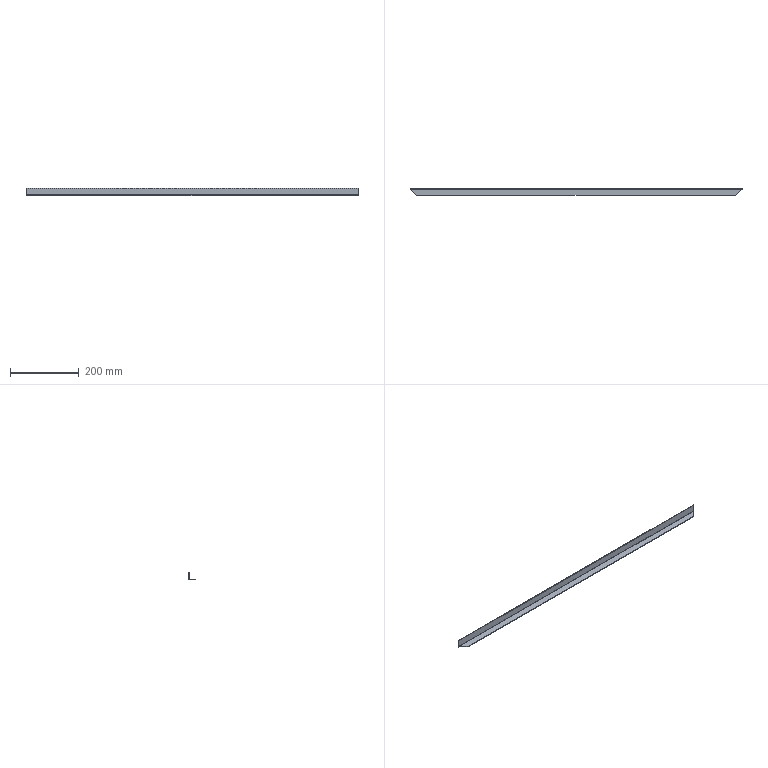Part | STEP file | Rear Closing Plate Frame Lower 1 | 1 solid | 22 faces | box 963 x 20 x 22 mm | volume 74999 mm3 | plane 18 | cylinder 2 | spline 2 | commonest cylinder face diameters 1 x1 5 x1
STEP:
#1=CARTESIAN_POINT('',(-1.251,219.392,2.5));
#2=VERTEX_POINT('',#1);
#3=CARTESIAN_POINT('',(957.749,219.392,2.5));
#4=VERTEX_POINT('',#3);
#5=CARTESIAN_POINT('',(-3.251,219.392,2.5));
#6=DIRECTION('',(1.,0.,0.));
#7=VECTOR('',#6,1000.);
#8=LINE('',#5,#7);
#9=EDGE_CURVE('',#2,#4,#8,.T.);
#10=ORIENTED_EDGE('',*,*,#9,.F.);
#11=CARTESIAN_POINT('',(-1.251,219.392,3.5));
#12=VERTEX_POINT('',#11);
#13=CARTESIAN_POINT('',(-1.251,219.392,22.));
#14=DIRECTION('',(0.,0.,1.));
#15=VECTOR('',#14,1000.);
#16=LINE('',#13,#15);
#17=EDGE_CURVE('',#2,#12,#16,.T.);
#18=ORIENTED_EDGE('',*,*,#17,.T.);
#19=CARTESIAN_POINT('',(-2.251,219.392,3.5));
#20=VERTEX_POINT('',#19);
#21=CARTESIAN_POINT('',(-3.251,219.392,3.5));
#22=DIRECTION('',(-1.,0.,0.));
#23=VECTOR('',#22,1000.);
#24=LINE('',#21,#23);
#25=EDGE_CURVE('',#12,#20,#24,.T.);
#26=ORIENTED_EDGE('',*,*,#25,.T.);
#27=CARTESIAN_POINT('',(-2.251,219.392,0.));
#28=VERTEX_POINT('',#27);
#29=CARTESIAN_POINT('',(-2.251,219.392,22.));
#30=DIRECTION('',(0.,0.,1.));
#31=VECTOR('',#30,1000.);
#32=LINE('',#29,#31);
#33=EDGE_CURVE('',#28,#20,#32,.T.);
#34=ORIENTED_EDGE('',*,*,#33,.F.);
#35=CARTESIAN_POINT('',(-3.251,219.392,0.));
#36=VERTEX_POINT('',#35);
#37=CARTESIAN_POINT('',(-3.251,219.392,0.));
#38=DIRECTION('',(1.,0.,0.));
#39=VECTOR('',#38,1000.);
#40=LINE('',#37,#39);
#41=EDGE_CURVE('',#36,#28,#40,.T.);
#42=ORIENTED_EDGE('',*,*,#41,.F.);
#43=CARTESIAN_POINT('',(-3.251,219.392,22.));
#44=VERTEX_POINT('',#43);
#45=CARTESIAN_POINT('',(-3.251,219.392,22.));
#46=DIRECTION('',(0.,0.,-1.));
#47=VECTOR('',#46,1000.);
#48=LINE('',#45,#47);
#49=EDGE_CURVE('',#44,#36,#48,.T.);
#50=ORIENTED_EDGE('',*,*,#49,.F.);
#51=CARTESIAN_POINT('',(959.749,219.392,22.));
#52=VERTEX_POINT('',#51);
#53=CARTESIAN_POINT('',(-3.251,219.392,22.));
#54=DIRECTION('',(-1.,0.,0.));
#55=VECTOR('',#54,1000.);
#56=LINE('',#53,#55);
#57=EDGE_CURVE('',#52,#44,#56,.T.);
#58=ORIENTED_EDGE('',*,*,#57,.F.);
#59=CARTESIAN_POINT('',(959.749,219.392,0.));
#60=VERTEX_POINT('',#59);
#61=CARTESIAN_POINT('',(959.749,219.392,22.));
#62=DIRECTION('',(0.,0.,1.));
#63=VECTOR('',#62,1000.);
#64=LINE('',#61,#63);
#65=EDGE_CURVE('',#60,#52,#64,.T.);
#66=ORIENTED_EDGE('',*,*,#65,.F.);
#67=CARTESIAN_POINT('',(958.749,219.392,0.));
#68=VERTEX_POINT('',#67);
#69=CARTESIAN_POINT('',(959.749,219.392,0.));
#70=DIRECTION('',(1.,0.,0.));
#71=VECTOR('',#70,1000.);
#72=LINE('',#69,#71);
#73=EDGE_CURVE('',#68,#60,#72,.T.);
#74=ORIENTED_EDGE('',*,*,#73,.F.);
#75=CARTESIAN_POINT('',(958.749,219.392,3.5));
#76=VERTEX_POINT('',#75);
#77=CARTESIAN_POINT('',(958.749,219.392,22.));
#78=DIRECTION('',(0.,0.,-1.));
#79=VECTOR('',#78,1000.);
#80=LINE('',#77,#79);
#81=EDGE_CURVE('',#76,#68,#80,.T.);
#82=ORIENTED_EDGE('',*,*,#81,.F.);
#83=CARTESIAN_POINT('',(957.749,219.392,3.5));
#84=VERTEX_POINT('',#83);
#85=CARTESIAN_POINT('',(-3.251,219.392,3.5));
#86=DIRECTION('',(-1.,0.,0.));
#87=VECTOR('',#86,1000.);
#88=LINE('',#85,#87);
#89=EDGE_CURVE('',#76,#84,#88,.T.);
#90=ORIENTED_EDGE('',*,*,#89,.T.);
#91=CARTESIAN_POINT('',(957.749,219.392,22.));
#92=DIRECTION('',(0.,0.,-1.));
#93=VECTOR('',#92,1000.);
#94=LINE('',#91,#93);
#95=EDGE_CURVE('',#84,#4,#94,.T.);
#96=ORIENTED_EDGE('',*,*,#95,.T.);
#97=EDGE_LOOP('',(#10,#18,#26,#34,#42,#50,#58,#66,#74,#82,#90,#96));
#98=FACE_OUTER_BOUND('',#97,.T.);
#99=CARTESIAN_POINT('',(-3.251,219.392,22.));
#100=DIRECTION('',(0.,-1.,0.));
#101=DIRECTION('',(1.,0.,0.));
#102=AXIS2_PLACEMENT_3D('',#99,#100,#101);
#103=PLANE('',#102);
#104=ADVANCED_FACE('',(#98),#103,.F.);
#105=CARTESIAN_POINT('',(957.749,218.142,0.3349));
#106=VERTEX_POINT('',#105);
#107=CARTESIAN_POINT('',(957.749,216.892,2.5));
#108=DIRECTION('',(-1.,0.,0.));
#109=DIRECTION('',(0.,0.,1.));
#110=AXIS2_PLACEMENT_3D('',#107,#108,#109);
#111=CIRCLE('',#110,2.5);
#112=EDGE_CURVE('',#4,#106,#111,.T.);
#113=ORIENTED_EDGE('',*,*,#112,.T.);
#114=CARTESIAN_POINT('',(957.249,216.892,0.));
#115=VERTEX_POINT('',#114);
#116=CARTESIAN_POINT('',(957.249,216.892,0.));
#117=CARTESIAN_POINT('',(957.332,217.11,0.));
#118=CARTESIAN_POINT('',(957.416,217.328,0.02876));
#119=CARTESIAN_POINT('',(957.583,217.751,0.1422));
#120=CARTESIAN_POINT('',(957.665,217.952,0.2255));
#121=CARTESIAN_POINT('',(957.749,218.142,0.3349));
#122=B_SPLINE_CURVE_WITH_KNOTS('',3,(#116,#117,#118,#119,#120,#121),.UNSPECIFIED.,.F.,.F.,(4,2,4),(0.,0.0007013,0.001403),.UNSPECIFIED.);
#123=EDGE_CURVE('',#115,#106,#122,.T.);
#124=ORIENTED_EDGE('',*,*,#123,.F.);
#125=CARTESIAN_POINT('',(-0.7512,216.892,0.));
#126=VERTEX_POINT('',#125);
#127=CARTESIAN_POINT('',(1921.52,216.892,0.));
#128=DIRECTION('',(-1.,0.,0.));
#129=VECTOR('',#128,1000.);
#130=LINE('',#127,#129);
#131=EDGE_CURVE('',#115,#126,#130,.T.);
#132=ORIENTED_EDGE('',*,*,#131,.T.);
#133=CARTESIAN_POINT('',(-1.251,218.142,0.3349));
#134=VERTEX_POINT('',#133);
#135=CARTESIAN_POINT('',(-1.251,218.142,0.3349));
#136=CARTESIAN_POINT('',(-1.168,217.952,0.2255));
#137=CARTESIAN_POINT('',(-1.084,217.749,0.1414));
#138=CARTESIAN_POINT('',(-0.9172,217.326,0.02839));
#139=CARTESIAN_POINT('',(-0.8347,217.11,0.));
#140=CARTESIAN_POINT('',(-0.7512,216.892,0.));
#141=B_SPLINE_CURVE_WITH_KNOTS('',3,(#135,#136,#137,#138,#139,#140),.UNSPECIFIED.,.F.,.F.,(4,2,4),(0.,0.0007013,0.001403),.UNSPECIFIED.);
#142=EDGE_CURVE('',#134,#126,#141,.T.);
#143=ORIENTED_EDGE('',*,*,#142,.F.);
#144=CARTESIAN_POINT('',(-1.251,216.892,2.5));
#145=DIRECTION('',(1.,0.,0.));
#146=DIRECTION('',(0.,0.,1.));
#147=AXIS2_PLACEMENT_3D('',#144,#145,#146);
#148=CIRCLE('',#147,2.5);
#149=EDGE_CURVE('',#134,#2,#148,.T.);
#150=ORIENTED_EDGE('',*,*,#149,.T.);
#151=ORIENTED_EDGE('',*,*,#9,.T.);
#152=EDGE_LOOP('',(#113,#124,#132,#143,#150,#151));
#153=FACE_OUTER_BOUND('',#152,.T.);
#154=CARTESIAN_POINT('',(1921.52,216.892,2.5));
#155=DIRECTION('',(-1.,0.,0.));
#156=DIRECTION('',(0.,0.,1.));
#157=AXIS2_PLACEMENT_3D('',#154,#155,#156);
#158=CYLINDRICAL_SURFACE('',#157,2.5);
#159=ADVANCED_FACE('',(#153),#158,.T.);
#160=ORIENTED_EDGE('',*,*,#33,.T.);
#161=CARTESIAN_POINT('',(-2.251,217.392,3.5));
#162=VERTEX_POINT('',#161);
#163=CARTESIAN_POINT('',(-2.251,-1709.111,3.5));
#164=DIRECTION('',(0.,1.,0.));
#165=VECTOR('',#164,1000.);
#166=LINE('',#163,#165);
#167=EDGE_CURVE('',#162,#20,#166,.T.);
#168=ORIENTED_EDGE('',*,*,#167,.F.);
#169=CARTESIAN_POINT('',(-2.251,217.392,0.));
#170=VERTEX_POINT('',#169);
#171=CARTESIAN_POINT('',(-2.251,217.392,22.));
#172=DIRECTION('',(0.,0.,1.));
#173=VECTOR('',#172,1000.);
#174=LINE('',#171,#173);
#175=EDGE_CURVE('',#170,#162,#174,.T.);
#176=ORIENTED_EDGE('',*,*,#175,.F.);
#177=CARTESIAN_POINT('',(-2.251,-1709.111,0.));
#178=DIRECTION('',(0.,-1.,0.));
#179=VECTOR('',#178,1000.);
#180=LINE('',#177,#179);
#181=EDGE_CURVE('',#28,#170,#180,.T.);
#182=ORIENTED_EDGE('',*,*,#181,.F.);
#183=EDGE_LOOP('',(#160,#168,#176,#182));
#184=FACE_OUTER_BOUND('',#183,.T.);
#185=CARTESIAN_POINT('',(-2.251,-1709.111,22.));
#186=DIRECTION('',(-1.,0.,0.));
#187=DIRECTION('',(0.,0.,1.));
#188=AXIS2_PLACEMENT_3D('',#185,#186,#187);
#189=PLANE('',#188);
#190=ADVANCED_FACE('',(#184),#189,.F.);
#191=ORIENTED_EDGE('',*,*,#49,.T.);
#192=CARTESIAN_POINT('',(-3.251,217.392,0.));
#193=VERTEX_POINT('',#192);
#194=CARTESIAN_POINT('',(-3.251,-1709.111,0.));
#195=DIRECTION('',(0.,1.,0.));
#196=VECTOR('',#195,1000.);
#197=LINE('',#194,#196);
#198=EDGE_CURVE('',#193,#36,#197,.T.);
#199=ORIENTED_EDGE('',*,*,#198,.F.);
#200=CARTESIAN_POINT('',(-3.251,217.392,22.));
#201=VERTEX_POINT('',#200);
#202=CARTESIAN_POINT('',(-3.251,217.392,22.));
#203=DIRECTION('',(0.,0.,-1.));
#204=VECTOR('',#203,1000.);
#205=LINE('',#202,#204);
#206=EDGE_CURVE('',#201,#193,#205,.T.);
#207=ORIENTED_EDGE('',*,*,#206,.F.);
#208=CARTESIAN_POINT('',(-3.251,-1709.111,22.));
#209=DIRECTION('',(0.,-1.,0.));
#210=VECTOR('',#209,1000.);
#211=LINE('',#208,#210);
#212=EDGE_CURVE('',#44,#201,#211,.T.);
#213=ORIENTED_EDGE('',*,*,#212,.F.);
#214=EDGE_LOOP('',(#191,#199,#207,#213));
#215=FACE_OUTER_BOUND('',#214,.T.);
#216=CARTESIAN_POINT('',(-3.251,-1709.111,22.));
#217=DIRECTION('',(1.,0.,0.));
#218=DIRECTION('',(0.,0.,-1.));
#219=AXIS2_PLACEMENT_3D('',#216,#217,#218);
#220=PLANE('',#219);
#221=ADVANCED_FACE('',(#215),#220,.F.);
#222=ORIENTED_EDGE('',*,*,#57,.T.);
#223=ORIENTED_EDGE('',*,*,#212,.T.);
#224=CARTESIAN_POINT('',(959.749,217.392,22.));
#225=VERTEX_POINT('',#224);
#226=CARTESIAN_POINT('',(0.,217.392,22.));
#227=DIRECTION('',(-1.,0.,0.));
#228=VECTOR('',#227,1000.);
#229=LINE('',#226,#228);
#230=EDGE_CURVE('',#225,#201,#229,.T.);
#231=ORIENTED_EDGE('',*,*,#230,.F.);
#232=CARTESIAN_POINT('',(959.749,-1709.111,22.));
#233=DIRECTION('',(0.,-1.,0.));
#234=VECTOR('',#233,1000.);
#235=LINE('',#232,#234);
#236=EDGE_CURVE('',#52,#225,#235,.T.);
#237=ORIENTED_EDGE('',*,*,#236,.F.);
#238=EDGE_LOOP('',(#222,#223,#231,#237));
#239=FACE_OUTER_BOUND('',#238,.T.);
#240=CARTESIAN_POINT('',(0.,-1709.111,22.));
#241=DIRECTION('',(0.,0.,-1.));
#242=DIRECTION('',(-1.,0.,0.));
#243=AXIS2_PLACEMENT_3D('',#240,#241,#242);
#244=PLANE('',#243);
#245=ADVANCED_FACE('',(#239),#244,.F.);
#246=CARTESIAN_POINT('',(959.749,217.392,0.));
#247=VERTEX_POINT('',#246);
#248=CARTESIAN_POINT('',(959.749,217.392,22.));
#249=DIRECTION('',(0.,0.,-1.));
#250=VECTOR('',#249,1000.);
#251=LINE('',#248,#250);
#252=EDGE_CURVE('',#225,#247,#251,.T.);
#253=ORIENTED_EDGE('',*,*,#252,.T.);
#254=CARTESIAN_POINT('',(959.749,-1709.111,0.));
#255=DIRECTION('',(0.,1.,0.));
#256=VECTOR('',#255,1000.);
#257=LINE('',#254,#256);
#258=EDGE_CURVE('',#247,#60,#257,.T.);
#259=ORIENTED_EDGE('',*,*,#258,.T.);
#260=ORIENTED_EDGE('',*,*,#65,.T.);
#261=ORIENTED_EDGE('',*,*,#236,.T.);
#262=EDGE_LOOP('',(#253,#259,#260,#261));
#263=FACE_OUTER_BOUND('',#262,.T.);
#264=CARTESIAN_POINT('',(959.749,-1709.111,22.));
#265=DIRECTION('',(1.,0.,0.));
#266=DIRECTION('',(0.,0.,-1.));
#267=AXIS2_PLACEMENT_3D('',#264,#265,#266);
#268=PLANE('',#267);
#269=ADVANCED_FACE('',(#263),#268,.T.);
#270=ORIENTED_EDGE('',*,*,#81,.T.);
#271=CARTESIAN_POINT('',(958.749,217.392,0.));
#272=VERTEX_POINT('',#271);
#273=CARTESIAN_POINT('',(958.749,-1709.111,0.));
#274=DIRECTION('',(0.,1.,0.));
#275=VECTOR('',#274,1000.);
#276=LINE('',#273,#275);
#277=EDGE_CURVE('',#272,#68,#276,.T.);
#278=ORIENTED_EDGE('',*,*,#277,.F.);
#279=CARTESIAN_POINT('',(958.749,217.392,3.5));
#280=VERTEX_POINT('',#279);
#281=CARTESIAN_POINT('',(958.749,217.392,22.));
#282=DIRECTION('',(0.,0.,-1.));
#283=VECTOR('',#282,1000.);
#284=LINE('',#281,#283);
#285=EDGE_CURVE('',#280,#272,#284,.T.);
#286=ORIENTED_EDGE('',*,*,#285,.F.);
#287=CARTESIAN_POINT('',(958.749,-1709.111,3.5));
#288=DIRECTION('',(0.,-1.,0.));
#289=VECTOR('',#288,1000.);
#290=LINE('',#287,#289);
#291=EDGE_CURVE('',#76,#280,#290,.T.);
#292=ORIENTED_EDGE('',*,*,#291,.F.);
#293=EDGE_LOOP('',(#270,#278,#286,#292));
#294=FACE_OUTER_BOUND('',#293,.T.);
#295=CARTESIAN_POINT('',(958.749,-1709.111,22.));
#296=DIRECTION('',(1.,0.,0.));
#297=DIRECTION('',(0.,0.,-1.));
#298=AXIS2_PLACEMENT_3D('',#295,#296,#297);
#299=PLANE('',#298);
#300=ADVANCED_FACE('',(#294),#299,.F.);
#301=CARTESIAN_POINT('',(957.749,217.142,2.067));
#302=VERTEX_POINT('',#301);
#303=CARTESIAN_POINT('',(957.749,217.142,2.067));
#304=DIRECTION('',(0.,0.5,-0.866));
#305=VECTOR('',#304,1000.);
#306=LINE('',#303,#305);
#307=EDGE_CURVE('',#302,#106,#306,.T.);
#308=ORIENTED_EDGE('',*,*,#307,.T.);
#309=ORIENTED_EDGE('',*,*,#112,.F.);
#310=ORIENTED_EDGE('',*,*,#95,.F.);
#311=CARTESIAN_POINT('',(957.749,217.392,3.5));
#312=VERTEX_POINT('',#311);
#313=CARTESIAN_POINT('',(957.749,-1709.111,3.5));
#314=DIRECTION('',(0.,-1.,0.));
#315=VECTOR('',#314,1000.);
#316=LINE('',#313,#315);
#317=EDGE_CURVE('',#84,#312,#316,.T.);
#318=ORIENTED_EDGE('',*,*,#317,.T.);
#319=CARTESIAN_POINT('',(957.749,217.392,2.5));
#320=VERTEX_POINT('',#319);
#321=CARTESIAN_POINT('',(957.749,217.392,22.));
#322=DIRECTION('',(0.,0.,1.));
#323=VECTOR('',#322,1000.);
#324=LINE('',#321,#323);
#325=EDGE_CURVE('',#320,#312,#324,.T.);
#326=ORIENTED_EDGE('',*,*,#325,.F.);
#327=CARTESIAN_POINT('',(957.749,216.892,2.5));
#328=DIRECTION('',(-1.,0.,0.));
#329=DIRECTION('',(0.,0.,1.));
#330=AXIS2_PLACEMENT_3D('',#327,#328,#329);
#331=CIRCLE('',#330,0.5);
#332=EDGE_CURVE('',#320,#302,#331,.T.);
#333=ORIENTED_EDGE('',*,*,#332,.T.);
#334=EDGE_LOOP('',(#308,#309,#310,#318,#326,#333));
#335=FACE_OUTER_BOUND('',#334,.T.);
#336=CARTESIAN_POINT('',(957.749,216.892,2.5));
#337=DIRECTION('',(1.,0.,0.));
#338=DIRECTION('',(0.,0.,-1.));
#339=AXIS2_PLACEMENT_3D('',#336,#337,#338);
#340=PLANE('',#339);
#341=ADVANCED_FACE('',(#335),#340,.T.);
#342=CARTESIAN_POINT('',(-1.251,217.142,2.067));
#343=VERTEX_POINT('',#342);
#344=CARTESIAN_POINT('',(-1.251,217.392,2.5));
#345=VERTEX_POINT('',#344);
#346=CARTESIAN_POINT('',(-1.251,216.892,2.5));
#347=DIRECTION('',(1.,0.,0.));
#348=DIRECTION('',(0.,0.,1.));
#349=AXIS2_PLACEMENT_3D('',#346,#347,#348);
#350=CIRCLE('',#349,0.5);
#351=EDGE_CURVE('',#343,#345,#350,.T.);
#352=ORIENTED_EDGE('',*,*,#351,.T.);
#353=CARTESIAN_POINT('',(-1.251,217.392,3.5));
#354=VERTEX_POINT('',#353);
#355=CARTESIAN_POINT('',(-1.251,217.392,22.));
#356=DIRECTION('',(0.,0.,-1.));
#357=VECTOR('',#356,1000.);
#358=LINE('',#355,#357);
#359=EDGE_CURVE('',#354,#345,#358,.T.);
#360=ORIENTED_EDGE('',*,*,#359,.F.);
#361=CARTESIAN_POINT('',(-1.251,-1709.111,3.5));
#362=DIRECTION('',(0.,1.,0.));
#363=VECTOR('',#362,1000.);
#364=LINE('',#361,#363);
#365=EDGE_CURVE('',#354,#12,#364,.T.);
#366=ORIENTED_EDGE('',*,*,#365,.T.);
#367=ORIENTED_EDGE('',*,*,#17,.F.);
#368=ORIENTED_EDGE('',*,*,#149,.F.);
#369=CARTESIAN_POINT('',(-1.251,218.142,0.3349));
#370=DIRECTION('',(0.,-0.5,0.866));
#371=VECTOR('',#370,1000.);
#372=LINE('',#369,#371);
#373=EDGE_CURVE('',#134,#343,#372,.T.);
#374=ORIENTED_EDGE('',*,*,#373,.T.);
#375=EDGE_LOOP('',(#352,#360,#366,#367,#368,#374));
#376=FACE_OUTER_BOUND('',#375,.T.);
#377=CARTESIAN_POINT('',(-1.251,216.892,2.5));
#378=DIRECTION('',(-1.,0.,0.));
#379=DIRECTION('',(0.,0.,1.));
#380=AXIS2_PLACEMENT_3D('',#377,#378,#379);
#381=PLANE('',#380);
#382=ADVANCED_FACE('',(#376),#381,.T.);
#383=CARTESIAN_POINT('',(939.749,199.392,0.));
#384=VERTEX_POINT('',#383);
#385=CARTESIAN_POINT('',(957.249,216.892,0.));
#386=DIRECTION('',(-0.7071,-0.7071,0.));
#387=VECTOR('',#386,1000.);
#388=LINE('',#385,#387);
#389=EDGE_CURVE('',#115,#384,#388,.T.);
#390=ORIENTED_EDGE('',*,*,#389,.T.);
#391=CARTESIAN_POINT('',(16.749,199.392,0.));
#392=VERTEX_POINT('',#391);
#393=CARTESIAN_POINT('',(0.,199.392,0.));
#394=DIRECTION('',(-1.,0.,0.));
#395=VECTOR('',#394,1000.);
#396=LINE('',#393,#395);
#397=EDGE_CURVE('',#384,#392,#396,.T.);
#398=ORIENTED_EDGE('',*,*,#397,.T.);
#399=CARTESIAN_POINT('',(16.749,199.392,0.));
#400=DIRECTION('',(-0.7071,0.7071,0.));
#401=VECTOR('',#400,1000.);
#402=LINE('',#399,#401);
#403=EDGE_CURVE('',#392,#126,#402,.T.);
#404=ORIENTED_EDGE('',*,*,#403,.T.);
#405=ORIENTED_EDGE('',*,*,#131,.F.);
#406=EDGE_LOOP('',(#390,#398,#404,#405));
#407=FACE_OUTER_BOUND('',#406,.T.);
#408=CARTESIAN_POINT('',(0.,0.,0.));
#409=DIRECTION('',(0.,0.,-1.));
#410=DIRECTION('',(-1.,0.,0.));
#411=AXIS2_PLACEMENT_3D('',#408,#409,#410);
#412=PLANE('',#411);
#413=ADVANCED_FACE('',(#407),#412,.T.);
#414=CARTESIAN_POINT('',(-3.251,217.392,0.));
#415=DIRECTION('',(-1.,0.,0.));
#416=VECTOR('',#415,1000.);
#417=LINE('',#414,#416);
#418=EDGE_CURVE('',#170,#193,#417,.T.);
#419=ORIENTED_EDGE('',*,*,#418,.T.);
#420=ORIENTED_EDGE('',*,*,#198,.T.);
#421=ORIENTED_EDGE('',*,*,#41,.T.);
#422=ORIENTED_EDGE('',*,*,#181,.T.);
#423=EDGE_LOOP('',(#419,#420,#421,#422));
#424=FACE_OUTER_BOUND('',#423,.T.);
#425=CARTESIAN_POINT('',(-3.251,-1709.111,0.));
#426=DIRECTION('',(0.,0.,-1.));
#427=DIRECTION('',(-1.,0.,0.));
#428=AXIS2_PLACEMENT_3D('',#425,#426,#427);
#429=PLANE('',#428);
#430=ADVANCED_FACE('',(#424),#429,.T.);
#431=ORIENTED_EDGE('',*,*,#25,.F.);
#432=ORIENTED_EDGE('',*,*,#365,.F.);
#433=CARTESIAN_POINT('',(-3.251,217.392,3.5));
#434=DIRECTION('',(1.,0.,0.));
#435=VECTOR('',#434,1000.);
#436=LINE('',#433,#435);
#437=EDGE_CURVE('',#162,#354,#436,.T.);
#438=ORIENTED_EDGE('',*,*,#437,.F.);
#439=ORIENTED_EDGE('',*,*,#167,.T.);
#440=EDGE_LOOP('',(#431,#432,#438,#439));
#441=FACE_OUTER_BOUND('',#440,.T.);
#442=CARTESIAN_POINT('',(-3.251,-1709.111,3.5));
#443=DIRECTION('',(0.,0.,1.));
#444=DIRECTION('',(1.,0.,0.));
#445=AXIS2_PLACEMENT_3D('',#442,#443,#444);
#446=PLANE('',#445);
#447=ADVANCED_FACE('',(#441),#446,.F.);
#448=ORIENTED_EDGE('',*,*,#437,.T.);
#449=ORIENTED_EDGE('',*,*,#359,.T.);
#450=CARTESIAN_POINT('',(-3.251,217.392,2.5));
#451=DIRECTION('',(1.,0.,0.));
#452=VECTOR('',#451,1000.);
#453=LINE('',#450,#452);
#454=EDGE_CURVE('',#345,#320,#453,.T.);
#455=ORIENTED_EDGE('',*,*,#454,.T.);
#456=ORIENTED_EDGE('',*,*,#325,.T.);
#457=CARTESIAN_POINT('',(-3.251,217.392,3.5));
#458=DIRECTION('',(1.,0.,0.));
#459=VECTOR('',#458,1000.);
#460=LINE('',#457,#459);
#461=EDGE_CURVE('',#312,#280,#460,.T.);
#462=ORIENTED_EDGE('',*,*,#461,.T.);
#463=ORIENTED_EDGE('',*,*,#285,.T.);
#464=CARTESIAN_POINT('',(-3.251,217.392,0.));
#465=DIRECTION('',(1.,0.,0.));
#466=VECTOR('',#465,1000.);
#467=LINE('',#464,#466);
#468=EDGE_CURVE('',#272,#247,#467,.T.);
#469=ORIENTED_EDGE('',*,*,#468,.T.);
#470=ORIENTED_EDGE('',*,*,#252,.F.);
#471=ORIENTED_EDGE('',*,*,#230,.T.);
#472=ORIENTED_EDGE('',*,*,#206,.T.);
#473=ORIENTED_EDGE('',*,*,#418,.F.);
#474=ORIENTED_EDGE('',*,*,#175,.T.);
#475=EDGE_LOOP('',(#448,#449,#455,#456,#462,#463,#469,#470,#471,#472,#473,#474));
#476=FACE_OUTER_BOUND('',#475,.T.);
#477=CARTESIAN_POINT('',(-3.251,217.392,22.));
#478=DIRECTION('',(0.,-1.,0.));
#479=DIRECTION('',(1.,0.,0.));
#480=AXIS2_PLACEMENT_3D('',#477,#478,#479);
#481=PLANE('',#480);
#482=ADVANCED_FACE('',(#476),#481,.T.);
#483=ORIENTED_EDGE('',*,*,#468,.F.);
#484=ORIENTED_EDGE('',*,*,#277,.T.);
#485=ORIENTED_EDGE('',*,*,#73,.T.);
#486=ORIENTED_EDGE('',*,*,#258,.F.);
#487=EDGE_LOOP('',(#483,#484,#485,#486));
#488=FACE_OUTER_BOUND('',#487,.T.);
#489=CARTESIAN_POINT('',(959.749,-1709.111,0.));
#490=DIRECTION('',(0.,0.,-1.));
#491=DIRECTION('',(-1.,0.,0.));
#492=AXIS2_PLACEMENT_3D('',#489,#490,#491);
#493=PLANE('',#492);
#494=ADVANCED_FACE('',(#488),#493,.T.);
#495=ORIENTED_EDGE('',*,*,#89,.F.);
#496=ORIENTED_EDGE('',*,*,#291,.T.);
#497=ORIENTED_EDGE('',*,*,#461,.F.);
#498=ORIENTED_EDGE('',*,*,#317,.F.);
#499=EDGE_LOOP('',(#495,#496,#497,#498));
#500=FACE_OUTER_BOUND('',#499,.T.);
#501=CARTESIAN_POINT('',(-3.251,-1709.111,3.5));
#502=DIRECTION('',(0.,0.,1.));
#503=DIRECTION('',(1.,0.,0.));
#504=AXIS2_PLACEMENT_3D('',#501,#502,#503);
#505=PLANE('',#504);
#506=ADVANCED_FACE('',(#500),#505,.F.);
#507=CARTESIAN_POINT('',(957.249,216.892,2.));
#508=VERTEX_POINT('',#507);
#509=CARTESIAN_POINT('',(957.249,216.892,1.));
#510=DIRECTION('',(0.,0.,-1.));
#511=VECTOR('',#510,1000.);
#512=LINE('',#509,#511);
#513=EDGE_CURVE('',#508,#115,#512,.T.);
#514=ORIENTED_EDGE('',*,*,#513,.T.);
#515=ORIENTED_EDGE('',*,*,#123,.T.);
#516=ORIENTED_EDGE('',*,*,#307,.F.);
#517=CARTESIAN_POINT('',(957.749,217.142,2.067));
#518=CARTESIAN_POINT('',(957.582,217.066,2.023));
#519=CARTESIAN_POINT('',(957.416,216.979,2.));
#520=CARTESIAN_POINT('',(957.249,216.892,2.));
#521=B_SPLINE_CURVE_WITH_KNOTS('',3,(#517,#518,#519,#520),.UNSPECIFIED.,.F.,.F.,(4,4),(0.,0.0005639),.UNSPECIFIED.);
#522=EDGE_CURVE('',#302,#508,#521,.T.);
#523=ORIENTED_EDGE('',*,*,#522,.T.);
#524=EDGE_LOOP('',(#514,#515,#516,#523));
#525=FACE_OUTER_BOUND('',#524,.T.);
#526=CARTESIAN_POINT('',(957.749,218.152,0.3176));
#527=CARTESIAN_POINT('',(957.582,217.77,0.09738));
#528=CARTESIAN_POINT('',(957.416,217.332,-0.02));
#529=CARTESIAN_POINT('',(957.249,216.892,-0.02));
#530=CARTESIAN_POINT('',(957.749,218.142,0.3349));
#531=CARTESIAN_POINT('',(957.582,217.763,0.1165));
#532=CARTESIAN_POINT('',(957.416,217.329,0.));
#533=CARTESIAN_POINT('',(957.249,216.892,0.));
#534=CARTESIAN_POINT('',(957.749,217.142,2.067));
#535=CARTESIAN_POINT('',(957.582,217.066,2.023));
#536=CARTESIAN_POINT('',(957.416,216.979,2.));
#537=CARTESIAN_POINT('',(957.249,216.892,2.));
#538=B_SPLINE_SURFACE_WITH_KNOTS('',1,3,((#526,#527,#528,#529),(#530,#531,#532,#533),(#534,#535,#536,#537)),.UNSPECIFIED.,.F.,.F.,.F.,(2,1,2),(4,4),(-0.01,0.,1.),(0.,1.),.UNSPECIFIED.);
#539=ADVANCED_FACE('',(#525),#538,.T.);
#540=ORIENTED_EDGE('',*,*,#142,.T.);
#541=CARTESIAN_POINT('',(-0.7512,216.892,2.));
#542=VERTEX_POINT('',#541);
#543=CARTESIAN_POINT('',(-0.7512,216.892,1.));
#544=DIRECTION('',(0.,0.,1.));
#545=VECTOR('',#544,1000.);
#546=LINE('',#543,#545);
#547=EDGE_CURVE('',#126,#542,#546,.T.);
#548=ORIENTED_EDGE('',*,*,#547,.T.);
#549=CARTESIAN_POINT('',(-0.7512,216.892,2.));
#550=CARTESIAN_POINT('',(-0.9179,216.979,2.));
#551=CARTESIAN_POINT('',(-1.084,217.066,2.023));
#552=CARTESIAN_POINT('',(-1.251,217.142,2.067));
#553=B_SPLINE_CURVE_WITH_KNOTS('',3,(#549,#550,#551,#552),.UNSPECIFIED.,.F.,.F.,(4,4),(0.,0.0005639),.UNSPECIFIED.);
#554=EDGE_CURVE('',#542,#343,#553,.T.);
#555=ORIENTED_EDGE('',*,*,#554,.T.);
#556=ORIENTED_EDGE('',*,*,#373,.F.);
#557=EDGE_LOOP('',(#540,#548,#555,#556));
#558=FACE_OUTER_BOUND('',#557,.T.);
#559=CARTESIAN_POINT('',(-0.7512,216.892,-0.02));
#560=CARTESIAN_POINT('',(-0.9181,217.332,-0.02));
#561=CARTESIAN_POINT('',(-1.084,217.77,0.09738));
#562=CARTESIAN_POINT('',(-1.251,218.152,0.3176));
#563=CARTESIAN_POINT('',(-0.7512,216.892,0.));
#564=CARTESIAN_POINT('',(-0.9181,217.329,0.));
#565=CARTESIAN_POINT('',(-1.084,217.763,0.1165));
#566=CARTESIAN_POINT('',(-1.251,218.142,0.3349));
#567=CARTESIAN_POINT('',(-0.7512,216.892,2.));
#568=CARTESIAN_POINT('',(-0.9179,216.979,2.));
#569=CARTESIAN_POINT('',(-1.084,217.066,2.023));
#570=CARTESIAN_POINT('',(-1.251,217.142,2.067));
#571=B_SPLINE_SURFACE_WITH_KNOTS('',1,3,((#559,#560,#561,#562),(#563,#564,#565,#566),(#567,#568,#569,#570)),.UNSPECIFIED.,.F.,.F.,.F.,(2,1,2),(4,4),(-0.01,0.,1.),(0.,1.),.UNSPECIFIED.);
#572=ADVANCED_FACE('',(#558),#571,.T.);
#573=CARTESIAN_POINT('',(939.749,199.392,2.));
#574=VERTEX_POINT('',#573);
#575=CARTESIAN_POINT('',(939.749,199.392,1918.32));
#576=DIRECTION('',(0.,0.,1.));
#577=VECTOR('',#576,1000.);
#578=LINE('',#575,#577);
#579=EDGE_CURVE('',#384,#574,#578,.T.);
#580=ORIENTED_EDGE('',*,*,#579,.T.);
#581=CARTESIAN_POINT('',(16.749,199.392,2.));
#582=VERTEX_POINT('',#581);
#583=CARTESIAN_POINT('',(0.,199.392,2.));
#584=DIRECTION('',(-1.,0.,0.));
#585=VECTOR('',#584,1000.);
#586=LINE('',#583,#585);
#587=EDGE_CURVE('',#574,#582,#586,.T.);
#588=ORIENTED_EDGE('',*,*,#587,.T.);
#589=CARTESIAN_POINT('',(16.749,199.392,1918.32));
#590=DIRECTION('',(0.,0.,-1.));
#591=VECTOR('',#590,1000.);
#592=LINE('',#589,#591);
#593=EDGE_CURVE('',#582,#392,#592,.T.);
#594=ORIENTED_EDGE('',*,*,#593,.T.);
#595=ORIENTED_EDGE('',*,*,#397,.F.);
#596=EDGE_LOOP('',(#580,#588,#594,#595));
#597=FACE_OUTER_BOUND('',#596,.T.);
#598=CARTESIAN_POINT('',(0.,199.392,1918.32));
#599=DIRECTION('',(0.,-1.,0.));
#600=DIRECTION('',(0.,0.,-1.));
#601=AXIS2_PLACEMENT_3D('',#598,#599,#600);
#602=PLANE('',#601);
#603=ADVANCED_FACE('',(#597),#602,.T.);
#604=ORIENTED_EDGE('',*,*,#513,.F.);
#605=CARTESIAN_POINT('',(370.179,-370.179,2.));
#606=DIRECTION('',(-0.7071,-0.7071,0.));
#607=VECTOR('',#606,1000.);
#608=LINE('',#605,#607);
#609=EDGE_CURVE('',#508,#574,#608,.T.);
#610=ORIENTED_EDGE('',*,*,#609,.T.);
#611=ORIENTED_EDGE('',*,*,#579,.F.);
#612=ORIENTED_EDGE('',*,*,#389,.F.);
#613=EDGE_LOOP('',(#604,#610,#611,#612));
#614=FACE_OUTER_BOUND('',#613,.T.);
#615=CARTESIAN_POINT('',(370.179,-370.179,1918.32));
#616=DIRECTION('',(0.7071,-0.7071,0.));
#617=DIRECTION('',(0.7071,0.7071,0.));
#618=AXIS2_PLACEMENT_3D('',#615,#616,#617);
#619=PLANE('',#618);
#620=ADVANCED_FACE('',(#614),#619,.T.);
#621=ORIENTED_EDGE('',*,*,#593,.F.);
#622=CARTESIAN_POINT('',(108.07,108.07,2.));
#623=DIRECTION('',(-0.7071,0.7071,0.));
#624=VECTOR('',#623,1000.);
#625=LINE('',#622,#624);
#626=EDGE_CURVE('',#582,#542,#625,.T.);
#627=ORIENTED_EDGE('',*,*,#626,.T.);
#628=ORIENTED_EDGE('',*,*,#547,.F.);
#629=ORIENTED_EDGE('',*,*,#403,.F.);
#630=EDGE_LOOP('',(#621,#627,#628,#629));
#631=FACE_OUTER_BOUND('',#630,.T.);
#632=CARTESIAN_POINT('',(108.07,108.07,1918.32));
#633=DIRECTION('',(-0.7071,-0.7071,0.));
#634=DIRECTION('',(0.7071,-0.7071,0.));
#635=AXIS2_PLACEMENT_3D('',#632,#633,#634);
#636=PLANE('',#635);
#637=ADVANCED_FACE('',(#631),#636,.T.);
#638=ORIENTED_EDGE('',*,*,#522,.F.);
#639=ORIENTED_EDGE('',*,*,#332,.F.);
#640=ORIENTED_EDGE('',*,*,#454,.F.);
#641=ORIENTED_EDGE('',*,*,#351,.F.);
#642=ORIENTED_EDGE('',*,*,#554,.F.);
#643=CARTESIAN_POINT('',(1921.52,216.892,2.));
#644=DIRECTION('',(-1.,0.,0.));
#645=VECTOR('',#644,1000.);
#646=LINE('',#643,#645);
#647=EDGE_CURVE('',#508,#542,#646,.T.);
#648=ORIENTED_EDGE('',*,*,#647,.F.);
#649=EDGE_LOOP('',(#638,#639,#640,#641,#642,#648));
#650=FACE_OUTER_BOUND('',#649,.T.);
#651=CARTESIAN_POINT('',(1921.52,216.892,2.5));
#652=DIRECTION('',(-1.,0.,0.));
#653=DIRECTION('',(0.,0.,1.));
#654=AXIS2_PLACEMENT_3D('',#651,#652,#653);
#655=CYLINDRICAL_SURFACE('',#654,0.5);
#656=ADVANCED_FACE('',(#650),#655,.F.);
#657=ORIENTED_EDGE('',*,*,#626,.F.);
#658=ORIENTED_EDGE('',*,*,#587,.F.);
#659=ORIENTED_EDGE('',*,*,#609,.F.);
#660=ORIENTED_EDGE('',*,*,#647,.T.);
#661=EDGE_LOOP('',(#657,#658,#659,#660));
#662=FACE_OUTER_BOUND('',#661,.T.);
#663=CARTESIAN_POINT('',(0.,0.,2.));
#664=DIRECTION('',(0.,0.,-1.));
#665=DIRECTION('',(-1.,0.,0.));
#666=AXIS2_PLACEMENT_3D('',#663,#664,#665);
#667=PLANE('',#666);
#668=ADVANCED_FACE('',(#662),#667,.F.);
#669=CLOSED_SHELL('',(#104,#159,#190,#221,#245,#269,#300,#341,#382,#413,#430,#447,#482,#494,#506,#539,#572,#603,#620,#637,#656,#668));
#670=MANIFOLD_SOLID_BREP('',#669);
#671=CARTESIAN_POINT('',(0.,0.,0.));
#672=DIRECTION('',(0.,0.,1.));
#673=DIRECTION('',(1.,0.,0.));
#674=AXIS2_PLACEMENT_3D('',#671,#672,#673);
#675=(LENGTH_UNIT()NAMED_UNIT(*)SI_UNIT(.MILLI.,.METRE.));
#676=UNCERTAINTY_MEASURE_WITH_UNIT(LENGTH_MEASURE(0.00001),#675,'','');
#677=(NAMED_UNIT(*)PLANE_ANGLE_UNIT()SI_UNIT($,.RADIAN.));
#678=(NAMED_UNIT(*)SI_UNIT($,.STERADIAN.)SOLID_ANGLE_UNIT());
#679=(GEOMETRIC_REPRESENTATION_CONTEXT(3)GLOBAL_UNCERTAINTY_ASSIGNED_CONTEXT((#676))GLOBAL_UNIT_ASSIGNED_CONTEXT((#675,#677,#678))REPRESENTATION_CONTEXT('',''));
#680=ADVANCED_BREP_SHAPE_REPRESENTATION('',(#670,#674),#679);